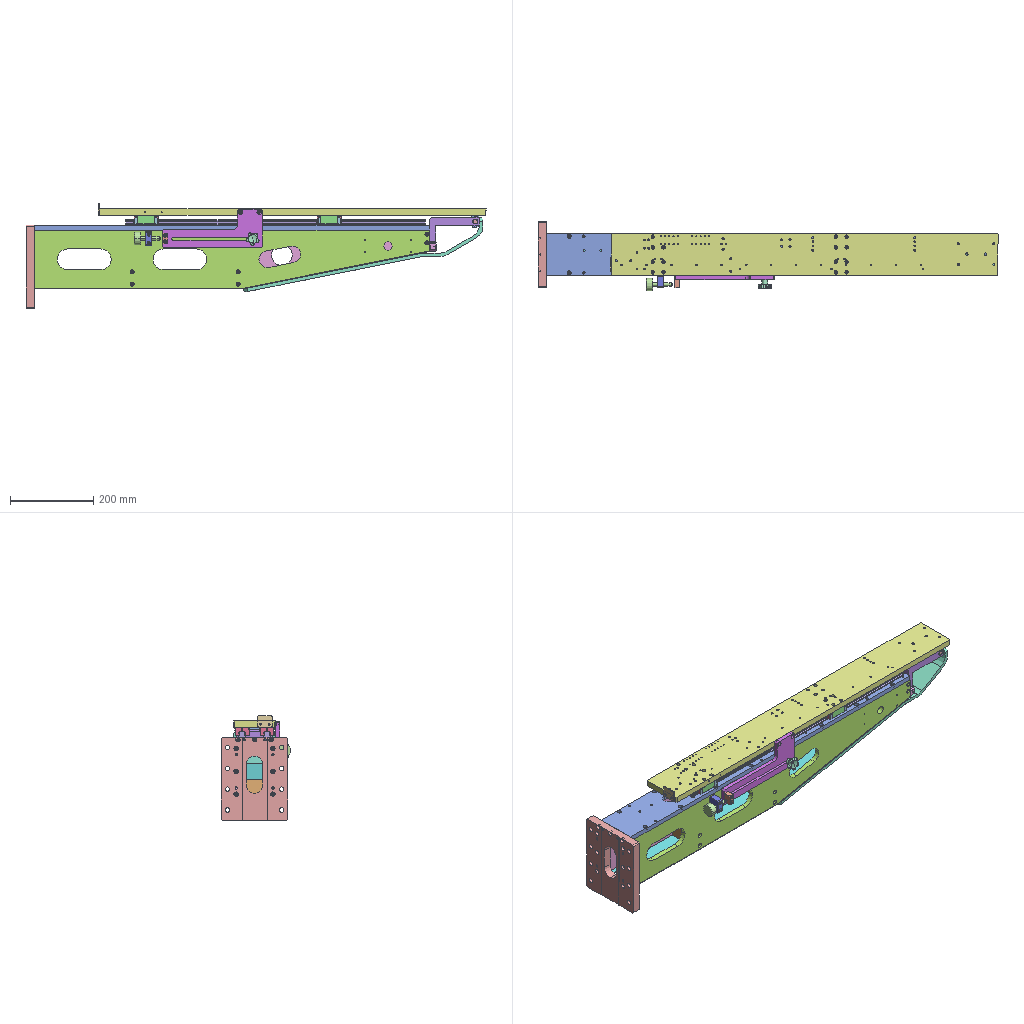Assembly | SolidWorks | 28 different items | 52 placed | box 1106 x 167 x 252 mm
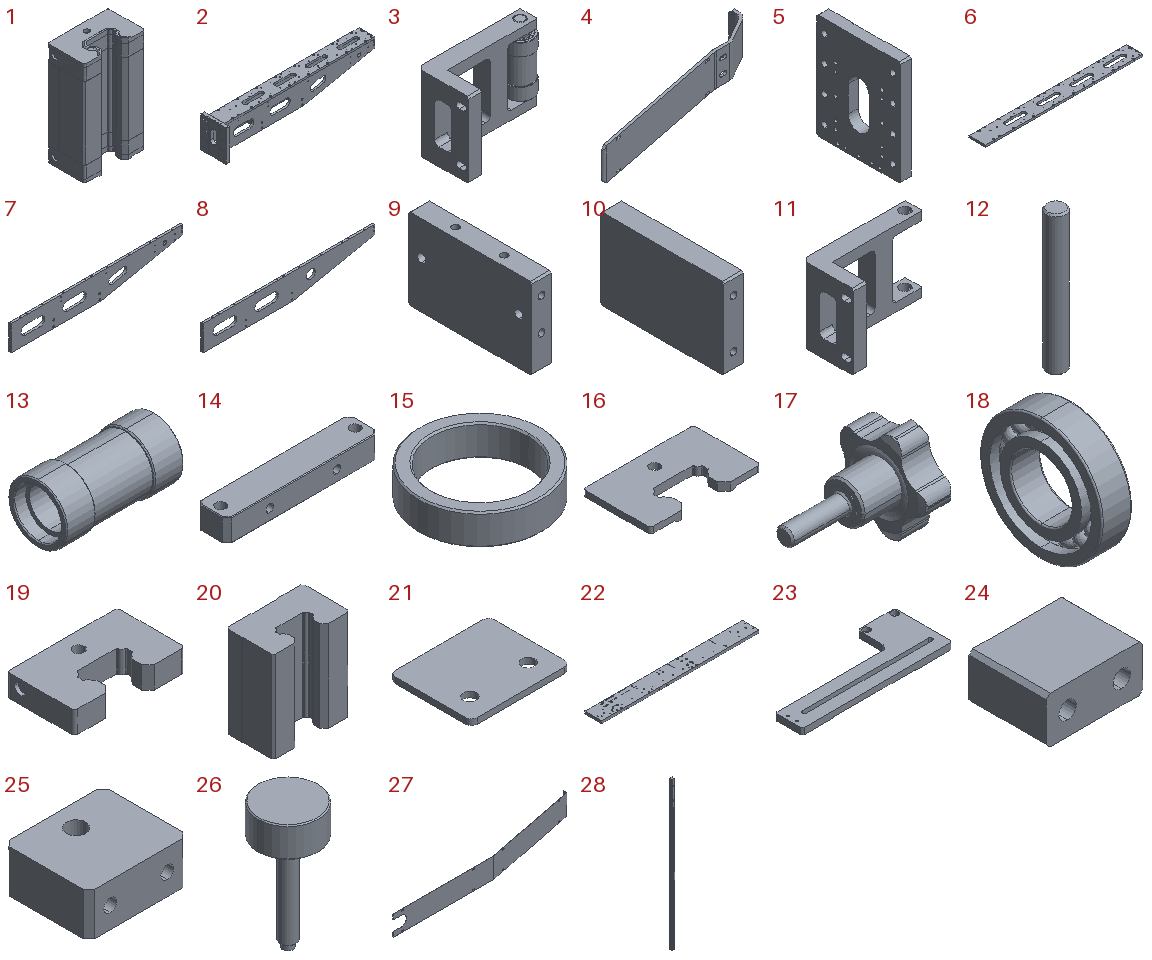Parts list (item | name | quantity | parent item | size | volume | features):
1 | (subassembly) | x4 | - | 34 x 21 x 58.6 mm | 32343 mm3 | -
2 | (subassembly) | x1 | - | 970 x 160 x 200 mm | 3941327 mm3 | features AEMSimFeature 1
3 | (subassembly) | x1 | - | 125 x 65 x 88 mm | 172222 mm3 | features AEMSimFeature 1
4 | - | x1 | - | 576.058 x 178.723 x 100 mm | 494950 mm3 | features ICE 3, Fillet 2, Chamfer 1, ExtruThin 1
5 | - | x1 | in 2 | 20 x 160 x 200 mm | 537437 mm3 | features HoleWzd 2, ICE 2, Chamfer 1
6 | - | x1 | in 2 | 950 x 100 x 12 mm | 942474 mm3 | features HoleWzd 9, LPattern 3, Chamfer 1, Extrusion 1, ICE 1
7 | - | x1 | in 2 | 950 x 12 x 140 mm | 1151524 mm3 | features HoleWzd 10, ICE 2, Chamfer 1
8 | - | x1 | in 2 | 950 x 12 x 140 mm | 1176953 mm3 | features HoleWzd 8, ICE 2, Chamfer 1
9 | - | x1 | in 2 | 12 x 76 x 50 mm | 43762 mm3 | features HoleWzd 3, Chamfer 1, ICE 1, MirrorPattern 1
10 | - | x2 | in 2 | 12 x 76 x 50 mm | 44588 mm3 | features HoleWzd 3, Chamfer 1, ICE 1, MirrorPattern 1
11 | - | x1 | in 3 | 120 x 60 x 88 mm | 139650 mm3 | features ICE 4, Chamfer 3, Extrusion 1, Fillet 1, HoleWzd 1
12 | - | x1 | in 3 | 12 x 12 x 88 mm | 9832 mm3 | features Chamfer 1, Extrusion 1, ICE 1, MirrorPattern 1
13 | - | x1 | in 3 | 60 x 30 x 30 mm | 19104 mm3 | features Chamfer 1, Revolution 1
14 | - | x1 | - | 100 x 20 x 15 mm | 27033 mm3 | features Chamfer 2, HoleWzd 2, Extrusion 1
15 | - | x2 | in 3 | 16 x 16 x 4 mm | 309.792 mm3 | features Chamfer 1, Extrusion 1
16 | - | x8 | in 1 | 33.5 x 20.5 x 2.5 mm | 1023 mm3 | features BaseBody 1
17 | - | x1 | - | 42.423 x 29.716 x 30.844 mm | 7689 mm3 | features BaseBody 1
18 | - | x2 | in 3 | 6 x 24 x 24 mm | 1508 mm3 | features Stock 1
19 | - | x8 | in 1 | 33.5 x 20.5 x 6.7 mm | 3669 mm3 | features BaseBody 1
20 | - | x4 | in 1 | 34 x 21 x 40.2 mm | 22959 mm3 | features BaseBody 1
21 | - | x1 | - | 34 x 28 x 2 mm | 1834 mm3 | features Extrusion 1, Fillet 1
22 | - | x1 | - | 930 x 100 x 15 mm | 1375215 mm3 | features HoleWzd 10, Chamfer 1, Extrusion 1, LPattern 1
23 | - | x1 | - | 240 x 92 x 10 mm | 112675 mm3 | features ICE 3, HoleWzd 2, Chamfer 1, Extrusion 1, Fillet 1
24 | - | x1 | - | 25 x 20 x 12 mm | 5021 mm3 | features Chamfer 1, Extrusion 1, HoleWzd 1
25 | - | x1 | - | 35 x 30 x 15 mm | 13829 mm3 | features HoleWzd 2, Chamfer 1, Extrusion 1
26 | - | x1 | - | 30 x 30 x 63 mm | 12897 mm3 | features ICE 3, Chamfer 1, Extrusion 1
27 | - | x1 | - | 946 x 108 x 100 mm | 93762 mm3 | features ICE 4, ExtruThin 1, Fillet 1
28 | - | x2 | - | 15 x 13 x 720 mm | 116945 mm3 | features Fillet 8, ICE 4, Chamfer 2, Extrusion 1, HoleWzd 1, LPattern 1
Mates (type | each side: item.copy, entity, surface, feature):
In the top assembly
Coincident | 28.1 face plane Boss-Extrude1 | 20.1 face plane Input1
Coincident | 28.1 face plane Cut-Extrude1 | 19.1 face plane Input1
Coincident | 28.2 face plane Boss-Extrude1 | 20.2 face plane Input1
Coincident | 28.2 face plane Cut-Extrude1 | 20.2 face plane Input1
Coincident | 16.1 face plane Input1 | 16.2 face plane Input1
Concentric | 20.1 face cylinder Input1 | 22.1 face cylinder Hole size per hex socket screw type1
Coincident | 20.1 face plane Input1 | 22.1 face plane Boss-Extrude1
Coincident | 22.1 face plane Boss-Extrude1 | 23.1 face plane Boss-Extrude1
Concentric | 22.1 face cylinder M6 Tapped Hole2 | 23.1 face cylinder CBORE for M6 Hex Socket Head Cap Screw1 | 2 times
Coincident | 23.1 face plane Boss-Extrude1 | 17.1 face plane Input1
Coincident | 23.1 face plane Boss-Extrude1 | 24.1 face plane Boss-Extrude1
Concentric | 23.1 face cylinder M4 Tapped Hole1 | 24.1 face cylinder CBORE for M4 Hex Socket Head Cap Screw1 | 2 times
Concentric | 25.1 face cylinder M8 Tapped Hole1 | 26.1 face cylinder Boss-Extrude1
Concentric | 20.3 face cylinder Input1 | 22.1 face cylinder Hole size per hex socket screw type1
Coincident | 22.1 face plane Boss-Extrude1 | 21.1 face plane Boss-Extrude1
Concentric | 22.1 face cylinder M4 Tapped Hole3 | 21.1 face cylinder Boss-Extrude1 | 2 times
Concentric | 7.1 face cylinder M4 Tapped Hole2 | 25.1 face cylinder CBORE for M4 Hex Socket Head Cap Screw1 | 2 times
Concentric | 7.1 face cylinder M6 Tapped Hole1 | 17.1 face cylinder Input1
Coincident | 6.1 face plane Boss-Extrude1 | 28.1 face plane Boss-Extrude1
Concentric | 6.1 face cylinder M4 Tapped Hole1 | 28.1 face cylinder Hole1
Concentric | 6.1 face cylinder M4 Tapped Hole1 | 28.2 face cylinder Hole1
Coincident | 6.1 face plane Boss-Extrude1 | 28.2 face plane Boss-Extrude1
Parallel | 6.1 face plane Boss-Extrude1 | 28.1 face plane Boss-Extrude1
Concentric | 7.1 face cylinder M6 Tapped Hole3 | 27.1 face cylinder Cut-Extrude1
Concentric | 8.1 face cylinder M6 Tapped Hole3 | 27.1 face cylinder Cut-Extrude1
Coincident | 8.1 face plane Boss-Extrude2 | 27.1 face plane Extrude-Thin1
Coincident | 9.1 face plane Boss-Extrude6 | 11.1 face plane Boss-Extrude1
DistanceDim | 11.1 face plane Boss-Extrude1 | 7.1 face plane Boss-Extrude2
Tangent | 22.1 face plane Boss-Extrude1 | 13.1 face cylinder Revolve1
Concentric | 7.1 face cylinder M6 Tapped Hole3 | 14.1 face cylinder Hole size per hex socket screw type1
Concentric | 8.1 face cylinder M6 Tapped Hole3 | 14.1 face cylinder Hole size per hex socket screw type1
Coincident | 27.1 face plane Extrude-Thin1 | 14.1 face plane Boss-Extrude1
Coincident | 7.1 face plane Boss-Extrude2 | 4.1 face plane Extrude-Thin1
Coincident | 11.1 face plane Boss-Extrude1 | 4.1 face plane Extrude-Thin1
In subassembly 2
Coincident | 5.1 face plane Boss-Extrude4 | 6.2 face plane Boss-Extrude1
Coincident | 5.1 face plane Boss-Extrude4 | 2.1 plane | 2 times
Coincident | 5.1 plane | 2.1 plane
Coincident | 5.1 face plane Boss-Extrude4 | 7.2 face plane Boss-Extrude2
Concentric | 5.1 face cylinder Hole size per hex socket screw type1 | 7.2 face cylinder M6 Tapped Hole2 | 2 times
Concentric | 5.1 face cylinder Hole size per hex socket screw type1 | 6.2 face cylinder M6 Tapped Hole1 | 2 times
Concentric | 5.1 face cylinder Hole size per hex socket screw type1 | 8.2 face cylinder M6 Tapped Hole2
Coincident | 5.1 face plane Boss-Extrude4 | 8.2 face plane Boss-Extrude2
Concentric | 6.2 face cylinder LPattern2 | 8.2 face cylinder M5 Tapped Hole1
Coincident | 7.2 face plane Boss-Extrude2 | 9.2 face plane Boss-Extrude6
Concentric | 7.2 face cylinder Hole size per hex socket screw type1 | 9.2 face cylinder M5 Tapped Hole3 | 2 times
Coincident | 8.2 face plane Boss-Extrude2 | 10.1 face plane Boss-Extrude6
Concentric | 8.2 face cylinder Hole size per hex socket screw type1 | 10.1 face cylinder Mirror1 | 2 times
Concentric | 7.2 face cylinder Hole size per hex socket screw type1 | 10.2 face cylinder M5 Tapped Hole3 | 2 times
Coincident | 7.2 face plane Boss-Extrude2 | 10.2 face plane Boss-Extrude6
In subassembly 3
Concentric | 13.2 face cylinder Revolve1 | 18.1 face cylinder deep groove ball bearings gb
Coincident | 13.2 face plane Revolve1 | 18.1 face plane deep groove ball bearings gb
Concentric | 13.2 face cylinder Revolve1 | 18.2 face cylinder deep groove ball bearings gb
Coincident | 13.2 face plane Revolve1 | 18.2 face plane deep groove ball bearings gb
Concentric | 12.1 face cylinder Boss-Extrude1 | 18.2 face cylinder deep groove ball bearings gb
Concentric | 15.1 face cylinder Boss-Extrude1 | 12.1 face cylinder Boss-Extrude1
Coincident | 15.1 face plane Boss-Extrude1 | 18.1 face plane deep groove ball bearings gb
Concentric | 12.1 face cylinder Boss-Extrude1 | 15.2 face cylinder Boss-Extrude1
Coincident | 18.2 face plane deep groove ball bearings gb | 15.2 face plane Boss-Extrude1
Concentric | 11.2 face cylinder Boss-Extrude1 | 12.1 face cylinder Boss-Extrude1
Coincident | 11.2 face plane Boss-Extrude1 | 12.1 face plane Boss-Extrude1
Coincident | 11.2 face plane Cut-Extrude1 | 15.2 face plane Boss-Extrude1